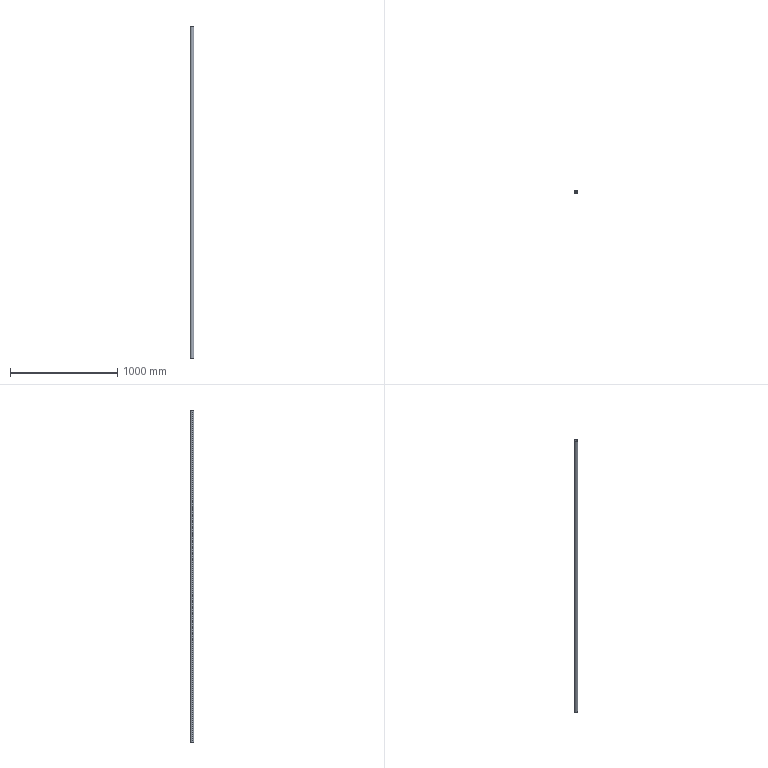Part | SolidWorks | features Extrusion 1 | 1 solid | 6 faces | box 32 x 32 x 3100 mm | volume 584336 mm3 | cylinder 4 | plane 2 | commonest cylinder face diameters 28 x2 32 x2
STEP:
#1=CARTESIAN_POINT('',(-14.,0.,1550.));
#2=VERTEX_POINT('',#1);
#3=CARTESIAN_POINT('',(14.,0.,1550.));
#4=VERTEX_POINT('',#3);
#5=CARTESIAN_POINT('',(0.,0.,1550.));
#6=DIRECTION('',(0.,0.,1.));
#7=DIRECTION('',(1.,0.,0.));
#8=AXIS2_PLACEMENT_3D('',#5,#6,#7);
#9=CIRCLE('',#8,14.);
#10=EDGE_CURVE('',#2,#4,#9,.T.);
#11=ORIENTED_EDGE('',*,*,#10,.T.);
#12=CARTESIAN_POINT('',(14.,0.,-1550.));
#13=VERTEX_POINT('',#12);
#14=CARTESIAN_POINT('',(14.,0.,1550.));
#15=DIRECTION('',(0.,0.,-1.));
#16=VECTOR('',#15,1000.);
#17=LINE('',#14,#16);
#18=EDGE_CURVE('',#4,#13,#17,.T.);
#19=ORIENTED_EDGE('',*,*,#18,.T.);
#20=CARTESIAN_POINT('',(-14.,0.,-1550.));
#21=VERTEX_POINT('',#20);
#22=CARTESIAN_POINT('',(0.,0.,-1550.));
#23=DIRECTION('',(0.,0.,1.));
#24=DIRECTION('',(1.,0.,0.));
#25=AXIS2_PLACEMENT_3D('',#22,#23,#24);
#26=CIRCLE('',#25,14.);
#27=EDGE_CURVE('',#21,#13,#26,.T.);
#28=ORIENTED_EDGE('',*,*,#27,.F.);
#29=CARTESIAN_POINT('',(-14.,0.,1550.));
#30=DIRECTION('',(0.,0.,-1.));
#31=VECTOR('',#30,1000.);
#32=LINE('',#29,#31);
#33=EDGE_CURVE('',#2,#21,#32,.T.);
#34=ORIENTED_EDGE('',*,*,#33,.F.);
#35=EDGE_LOOP('',(#11,#19,#28,#34));
#36=FACE_OUTER_BOUND('',#35,.T.);
#37=CARTESIAN_POINT('',(0.,0.,1550.));
#38=DIRECTION('',(0.,0.,-1.));
#39=DIRECTION('',(-1.,0.,0.));
#40=AXIS2_PLACEMENT_3D('',#37,#38,#39);
#41=CYLINDRICAL_SURFACE('',#40,14.);
#42=ADVANCED_FACE('',(#36),#41,.F.);
#43=CARTESIAN_POINT('',(16.,0.,1550.));
#44=VERTEX_POINT('',#43);
#45=CARTESIAN_POINT('',(-16.,0.,1550.));
#46=VERTEX_POINT('',#45);
#47=CARTESIAN_POINT('',(0.,0.,1550.));
#48=DIRECTION('',(0.,0.,1.));
#49=DIRECTION('',(1.,0.,0.));
#50=AXIS2_PLACEMENT_3D('',#47,#48,#49);
#51=CIRCLE('',#50,16.);
#52=EDGE_CURVE('',#44,#46,#51,.T.);
#53=ORIENTED_EDGE('',*,*,#52,.F.);
#54=CARTESIAN_POINT('',(16.,0.,-1550.));
#55=VERTEX_POINT('',#54);
#56=CARTESIAN_POINT('',(16.,0.,1550.));
#57=DIRECTION('',(0.,0.,-1.));
#58=VECTOR('',#57,1000.);
#59=LINE('',#56,#58);
#60=EDGE_CURVE('',#44,#55,#59,.T.);
#61=ORIENTED_EDGE('',*,*,#60,.T.);
#62=CARTESIAN_POINT('',(-16.,0.,-1550.));
#63=VERTEX_POINT('',#62);
#64=CARTESIAN_POINT('',(0.,0.,-1550.));
#65=DIRECTION('',(0.,0.,1.));
#66=DIRECTION('',(1.,0.,0.));
#67=AXIS2_PLACEMENT_3D('',#64,#65,#66);
#68=CIRCLE('',#67,16.);
#69=EDGE_CURVE('',#55,#63,#68,.T.);
#70=ORIENTED_EDGE('',*,*,#69,.T.);
#71=CARTESIAN_POINT('',(-16.,0.,1550.));
#72=DIRECTION('',(0.,0.,-1.));
#73=VECTOR('',#72,1000.);
#74=LINE('',#71,#73);
#75=EDGE_CURVE('',#46,#63,#74,.T.);
#76=ORIENTED_EDGE('',*,*,#75,.F.);
#77=EDGE_LOOP('',(#53,#61,#70,#76));
#78=FACE_OUTER_BOUND('',#77,.T.);
#79=CARTESIAN_POINT('',(0.,0.,1550.));
#80=DIRECTION('',(0.,0.,-1.));
#81=DIRECTION('',(-1.,0.,0.));
#82=AXIS2_PLACEMENT_3D('',#79,#80,#81);
#83=CYLINDRICAL_SURFACE('',#82,16.);
#84=ADVANCED_FACE('',(#78),#83,.T.);
#85=CARTESIAN_POINT('',(0.,0.,1550.));
#86=DIRECTION('',(0.,0.,1.));
#87=DIRECTION('',(1.,0.,0.));
#88=AXIS2_PLACEMENT_3D('',#85,#86,#87);
#89=CIRCLE('',#88,16.);
#90=EDGE_CURVE('',#46,#44,#89,.T.);
#91=ORIENTED_EDGE('',*,*,#90,.T.);
#92=ORIENTED_EDGE('',*,*,#52,.T.);
#93=EDGE_LOOP('',(#91,#92));
#94=FACE_OUTER_BOUND('',#93,.T.);
#95=ORIENTED_EDGE('',*,*,#10,.F.);
#96=CARTESIAN_POINT('',(0.,0.,1550.));
#97=DIRECTION('',(0.,0.,1.));
#98=DIRECTION('',(1.,0.,0.));
#99=AXIS2_PLACEMENT_3D('',#96,#97,#98);
#100=CIRCLE('',#99,14.);
#101=EDGE_CURVE('',#4,#2,#100,.T.);
#102=ORIENTED_EDGE('',*,*,#101,.F.);
#103=EDGE_LOOP('',(#95,#102));
#104=FACE_BOUND('',#103,.T.);
#105=CARTESIAN_POINT('',(0.,0.,1550.));
#106=DIRECTION('',(0.,0.,1.));
#107=DIRECTION('',(1.,0.,0.));
#108=AXIS2_PLACEMENT_3D('',#105,#106,#107);
#109=PLANE('',#108);
#110=ADVANCED_FACE('',(#94,#104),#109,.T.);
#111=CARTESIAN_POINT('',(0.,0.,-1550.));
#112=DIRECTION('',(0.,0.,1.));
#113=DIRECTION('',(1.,0.,0.));
#114=AXIS2_PLACEMENT_3D('',#111,#112,#113);
#115=CIRCLE('',#114,16.);
#116=EDGE_CURVE('',#63,#55,#115,.T.);
#117=ORIENTED_EDGE('',*,*,#116,.F.);
#118=ORIENTED_EDGE('',*,*,#69,.F.);
#119=EDGE_LOOP('',(#117,#118));
#120=FACE_OUTER_BOUND('',#119,.T.);
#121=ORIENTED_EDGE('',*,*,#27,.T.);
#122=CARTESIAN_POINT('',(0.,0.,-1550.));
#123=DIRECTION('',(0.,0.,1.));
#124=DIRECTION('',(1.,0.,0.));
#125=AXIS2_PLACEMENT_3D('',#122,#123,#124);
#126=CIRCLE('',#125,14.);
#127=EDGE_CURVE('',#13,#21,#126,.T.);
#128=ORIENTED_EDGE('',*,*,#127,.T.);
#129=EDGE_LOOP('',(#121,#128));
#130=FACE_BOUND('',#129,.T.);
#131=CARTESIAN_POINT('',(0.,0.,-1550.));
#132=DIRECTION('',(0.,0.,1.));
#133=DIRECTION('',(1.,0.,0.));
#134=AXIS2_PLACEMENT_3D('',#131,#132,#133);
#135=PLANE('',#134);
#136=ADVANCED_FACE('',(#120,#130),#135,.F.);
#137=ORIENTED_EDGE('',*,*,#60,.F.);
#138=ORIENTED_EDGE('',*,*,#90,.F.);
#139=ORIENTED_EDGE('',*,*,#75,.T.);
#140=ORIENTED_EDGE('',*,*,#116,.T.);
#141=EDGE_LOOP('',(#137,#138,#139,#140));
#142=FACE_OUTER_BOUND('',#141,.T.);
#143=CARTESIAN_POINT('',(0.,0.,1550.));
#144=DIRECTION('',(0.,0.,-1.));
#145=DIRECTION('',(-1.,0.,0.));
#146=AXIS2_PLACEMENT_3D('',#143,#144,#145);
#147=CYLINDRICAL_SURFACE('',#146,16.);
#148=ADVANCED_FACE('',(#142),#147,.T.);
#149=ORIENTED_EDGE('',*,*,#18,.F.);
#150=ORIENTED_EDGE('',*,*,#101,.T.);
#151=ORIENTED_EDGE('',*,*,#33,.T.);
#152=ORIENTED_EDGE('',*,*,#127,.F.);
#153=EDGE_LOOP('',(#149,#150,#151,#152));
#154=FACE_OUTER_BOUND('',#153,.T.);
#155=CARTESIAN_POINT('',(0.,0.,1550.));
#156=DIRECTION('',(0.,0.,-1.));
#157=DIRECTION('',(-1.,0.,0.));
#158=AXIS2_PLACEMENT_3D('',#155,#156,#157);
#159=CYLINDRICAL_SURFACE('',#158,14.);
#160=ADVANCED_FACE('',(#154),#159,.F.);
#161=CLOSED_SHELL('',(#42,#84,#110,#136,#148,#160));
#162=MANIFOLD_SOLID_BREP('',#161);
#163=CARTESIAN_POINT('',(0.,0.,0.));
#164=DIRECTION('',(0.,0.,1.));
#165=DIRECTION('',(1.,0.,0.));
#166=AXIS2_PLACEMENT_3D('',#163,#164,#165);
#167=(LENGTH_UNIT()NAMED_UNIT(*)SI_UNIT(.MILLI.,.METRE.));
#168=UNCERTAINTY_MEASURE_WITH_UNIT(LENGTH_MEASURE(0.00001),#167,'','');
#169=(NAMED_UNIT(*)PLANE_ANGLE_UNIT()SI_UNIT($,.RADIAN.));
#170=(NAMED_UNIT(*)SI_UNIT($,.STERADIAN.)SOLID_ANGLE_UNIT());
#171=(GEOMETRIC_REPRESENTATION_CONTEXT(3)GLOBAL_UNCERTAINTY_ASSIGNED_CONTEXT((#168))GLOBAL_UNIT_ASSIGNED_CONTEXT((#167,#169,#170))REPRESENTATION_CONTEXT('',''));
#172=ADVANCED_BREP_SHAPE_REPRESENTATION('',(#162,#166),#171);